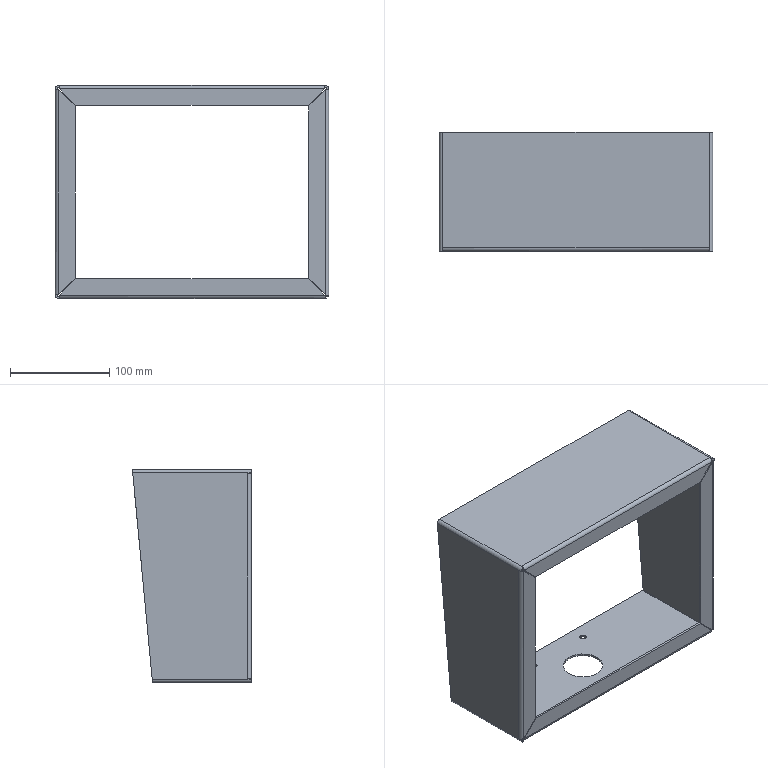Part | STEP file | Operation box SGN-7-03 | 1 solid | 80 faces | box 276 x 120 x 215 mm | volume 240191 mm3 | plane 46 | cylinder 24 | spline 10 | commonest cylinder face diameters 6.5 x8 3 x7 7 x7 40 x2